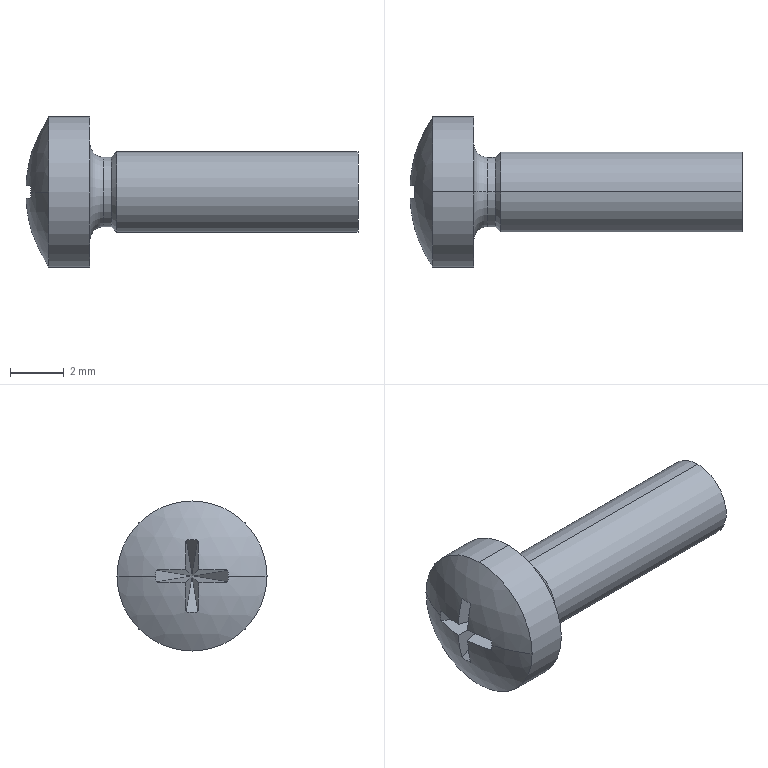Part | SolidWorks | features BaseBody 1 | 1 solid | 26 faces | box 12.388 x 5.6 x 5.6 mm | volume 116.992 mm3 | plane 14 | cylinder 6 | cone 2 | torus 2 | sphere 2 | commonest cylinder face diameters 2.598 x2 3 x2 5.6 x2
STEP:
#1=CARTESIAN_POINT('',(12.4,0.,1.5));
#2=VERTEX_POINT('',#1);
#3=CARTESIAN_POINT('',(12.4,0.,-1.5));
#4=VERTEX_POINT('',#3);
#5=CARTESIAN_POINT('',(12.4,0.,0.));
#6=DIRECTION('',(-1.,0.,0.));
#7=DIRECTION('',(0.,0.,1.));
#8=AXIS2_PLACEMENT_3D('',#5,#6,#7);
#9=CIRCLE('',#8,1.5);
#10=EDGE_CURVE('',#2,#4,#9,.T.);
#11=ORIENTED_EDGE('',*,*,#10,.T.);
#12=CARTESIAN_POINT('',(3.4,0.,-1.5));
#13=VERTEX_POINT('',#12);
#14=CARTESIAN_POINT('',(-1.332,0.,-1.5));
#15=DIRECTION('',(-1.,0.,0.));
#16=VECTOR('',#15,1000.);
#17=LINE('',#14,#16);
#18=EDGE_CURVE('',#4,#13,#17,.T.);
#19=ORIENTED_EDGE('',*,*,#18,.T.);
#20=CARTESIAN_POINT('',(3.4,0.,1.5));
#21=VERTEX_POINT('',#20);
#22=CARTESIAN_POINT('',(3.4,0.,0.));
#23=DIRECTION('',(-1.,0.,0.));
#24=DIRECTION('',(0.,0.,1.));
#25=AXIS2_PLACEMENT_3D('',#22,#23,#24);
#26=CIRCLE('',#25,1.5);
#27=EDGE_CURVE('',#21,#13,#26,.T.);
#28=ORIENTED_EDGE('',*,*,#27,.F.);
#29=CARTESIAN_POINT('',(-1.332,0.,1.5));
#30=DIRECTION('',(-1.,0.,0.));
#31=VECTOR('',#30,1000.);
#32=LINE('',#29,#31);
#33=EDGE_CURVE('',#2,#21,#32,.T.);
#34=ORIENTED_EDGE('',*,*,#33,.F.);
#35=EDGE_LOOP('',(#11,#19,#28,#34));
#36=FACE_OUTER_BOUND('',#35,.T.);
#37=CARTESIAN_POINT('',(-1.332,0.,0.));
#38=DIRECTION('',(-1.,0.,0.));
#39=DIRECTION('',(0.,0.,1.));
#40=AXIS2_PLACEMENT_3D('',#37,#38,#39);
#41=CYLINDRICAL_SURFACE('',#40,1.5);
#42=ADVANCED_FACE('',(#36),#41,.T.);
#43=CARTESIAN_POINT('',(3.199,0.,1.299));
#44=VERTEX_POINT('',#43);
#45=CARTESIAN_POINT('',(3.199,0.,-1.299));
#46=VERTEX_POINT('',#45);
#47=CARTESIAN_POINT('',(3.199,0.,0.));
#48=DIRECTION('',(-1.,0.,0.));
#49=DIRECTION('',(0.,0.,1.));
#50=AXIS2_PLACEMENT_3D('',#47,#48,#49);
#51=CIRCLE('',#50,1.299);
#52=EDGE_CURVE('',#44,#46,#51,.T.);
#53=ORIENTED_EDGE('',*,*,#52,.F.);
#54=CARTESIAN_POINT('',(3.4,0.,1.5));
#55=DIRECTION('',(0.7071,0.,0.7071));
#56=VECTOR('',#55,1000.);
#57=LINE('',#54,#56);
#58=EDGE_CURVE('',#44,#21,#57,.T.);
#59=ORIENTED_EDGE('',*,*,#58,.T.);
#60=ORIENTED_EDGE('',*,*,#27,.T.);
#61=CARTESIAN_POINT('',(3.4,0.,-1.5));
#62=DIRECTION('',(0.7071,0.,-0.7071));
#63=VECTOR('',#62,1000.);
#64=LINE('',#61,#63);
#65=EDGE_CURVE('',#46,#13,#64,.T.);
#66=ORIENTED_EDGE('',*,*,#65,.F.);
#67=EDGE_LOOP('',(#53,#59,#60,#66));
#68=FACE_OUTER_BOUND('',#67,.T.);
#69=CARTESIAN_POINT('',(3.4,0.,0.));
#70=DIRECTION('',(1.,0.,0.));
#71=DIRECTION('',(0.,0.,-1.));
#72=AXIS2_PLACEMENT_3D('',#69,#70,#71);
#73=CONICAL_SURFACE('',#72,1.5,0.7854);
#74=ADVANCED_FACE('',(#68),#73,.T.);
#75=ORIENTED_EDGE('',*,*,#52,.T.);
#76=CARTESIAN_POINT('',(2.901,0.,-1.299));
#77=VERTEX_POINT('',#76);
#78=CARTESIAN_POINT('',(-1.332,0.,-1.299));
#79=DIRECTION('',(-1.,0.,0.));
#80=VECTOR('',#79,1000.);
#81=LINE('',#78,#80);
#82=EDGE_CURVE('',#46,#77,#81,.T.);
#83=ORIENTED_EDGE('',*,*,#82,.T.);
#84=CARTESIAN_POINT('',(2.901,0.,1.299));
#85=VERTEX_POINT('',#84);
#86=CARTESIAN_POINT('',(2.901,0.,0.));
#87=DIRECTION('',(-1.,0.,0.));
#88=DIRECTION('',(0.,0.,1.));
#89=AXIS2_PLACEMENT_3D('',#86,#87,#88);
#90=CIRCLE('',#89,1.299);
#91=EDGE_CURVE('',#85,#77,#90,.T.);
#92=ORIENTED_EDGE('',*,*,#91,.F.);
#93=CARTESIAN_POINT('',(-1.332,0.,1.299));
#94=DIRECTION('',(-1.,0.,0.));
#95=VECTOR('',#94,1000.);
#96=LINE('',#93,#95);
#97=EDGE_CURVE('',#44,#85,#96,.T.);
#98=ORIENTED_EDGE('',*,*,#97,.F.);
#99=EDGE_LOOP('',(#75,#83,#92,#98));
#100=FACE_OUTER_BOUND('',#99,.T.);
#101=CARTESIAN_POINT('',(-1.332,0.,0.));
#102=DIRECTION('',(-1.,0.,0.));
#103=DIRECTION('',(0.,0.,1.));
#104=AXIS2_PLACEMENT_3D('',#101,#102,#103);
#105=CYLINDRICAL_SURFACE('',#104,1.299);
#106=ADVANCED_FACE('',(#100),#105,.T.);
#107=CARTESIAN_POINT('',(2.4,0.,-1.8));
#108=VERTEX_POINT('',#107);
#109=CARTESIAN_POINT('',(2.4,0.,1.8));
#110=VERTEX_POINT('',#109);
#111=CARTESIAN_POINT('',(2.4,0.,0.));
#112=DIRECTION('',(-1.,0.,0.));
#113=DIRECTION('',(0.,0.,1.));
#114=AXIS2_PLACEMENT_3D('',#111,#112,#113);
#115=CIRCLE('',#114,1.8);
#116=EDGE_CURVE('',#108,#110,#115,.T.);
#117=ORIENTED_EDGE('',*,*,#116,.F.);
#118=CARTESIAN_POINT('',(2.901,0.,-1.8));
#119=DIRECTION('',(0.,1.,0.));
#120=DIRECTION('',(0.,0.,1.));
#121=AXIS2_PLACEMENT_3D('',#118,#119,#120);
#122=CIRCLE('',#121,0.501);
#123=EDGE_CURVE('',#108,#77,#122,.T.);
#124=ORIENTED_EDGE('',*,*,#123,.T.);
#125=CARTESIAN_POINT('',(2.901,0.,0.));
#126=DIRECTION('',(-1.,0.,0.));
#127=DIRECTION('',(0.,0.,1.));
#128=AXIS2_PLACEMENT_3D('',#125,#126,#127);
#129=CIRCLE('',#128,1.299);
#130=EDGE_CURVE('',#77,#85,#129,.T.);
#131=ORIENTED_EDGE('',*,*,#130,.T.);
#132=CARTESIAN_POINT('',(2.901,0.,1.8));
#133=DIRECTION('',(0.,-1.,0.));
#134=DIRECTION('',(0.,0.,-1.));
#135=AXIS2_PLACEMENT_3D('',#132,#133,#134);
#136=CIRCLE('',#135,0.501);
#137=EDGE_CURVE('',#110,#85,#136,.T.);
#138=ORIENTED_EDGE('',*,*,#137,.F.);
#139=EDGE_LOOP('',(#117,#124,#131,#138));
#140=FACE_OUTER_BOUND('',#139,.T.);
#141=CARTESIAN_POINT('',(2.901,0.,0.));
#142=DIRECTION('',(-1.,0.,0.));
#143=DIRECTION('',(0.,0.,1.));
#144=AXIS2_PLACEMENT_3D('',#141,#142,#143);
#145=TOROIDAL_SURFACE('',#144,1.8,0.501);
#146=ADVANCED_FACE('',(#140),#145,.F.);
#147=CARTESIAN_POINT('',(2.4,0.,2.8));
#148=VERTEX_POINT('',#147);
#149=CARTESIAN_POINT('',(2.4,0.,-2.8));
#150=VERTEX_POINT('',#149);
#151=CARTESIAN_POINT('',(2.4,0.,0.));
#152=DIRECTION('',(-1.,0.,0.));
#153=DIRECTION('',(0.,0.,1.));
#154=AXIS2_PLACEMENT_3D('',#151,#152,#153);
#155=CIRCLE('',#154,2.8);
#156=EDGE_CURVE('',#148,#150,#155,.T.);
#157=ORIENTED_EDGE('',*,*,#156,.T.);
#158=CARTESIAN_POINT('',(0.8575,0.,-2.8));
#159=VERTEX_POINT('',#158);
#160=CARTESIAN_POINT('',(-1.332,0.,-2.8));
#161=DIRECTION('',(-1.,0.,0.));
#162=VECTOR('',#161,1000.);
#163=LINE('',#160,#162);
#164=EDGE_CURVE('',#150,#159,#163,.T.);
#165=ORIENTED_EDGE('',*,*,#164,.T.);
#166=CARTESIAN_POINT('',(0.8575,2.8,0.));
#167=VERTEX_POINT('',#166);
#168=CARTESIAN_POINT('',(0.8575,0.,0.));
#169=DIRECTION('',(-1.,0.,0.));
#170=DIRECTION('',(0.,0.,1.));
#171=AXIS2_PLACEMENT_3D('',#168,#169,#170);
#172=CIRCLE('',#171,2.8);
#173=EDGE_CURVE('',#167,#159,#172,.T.);
#174=ORIENTED_EDGE('',*,*,#173,.F.);
#175=CARTESIAN_POINT('',(0.8575,0.,2.8));
#176=VERTEX_POINT('',#175);
#177=CARTESIAN_POINT('',(0.8575,0.,0.));
#178=DIRECTION('',(-1.,0.,0.));
#179=DIRECTION('',(0.,0.,1.));
#180=AXIS2_PLACEMENT_3D('',#177,#178,#179);
#181=CIRCLE('',#180,2.8);
#182=EDGE_CURVE('',#176,#167,#181,.T.);
#183=ORIENTED_EDGE('',*,*,#182,.F.);
#184=CARTESIAN_POINT('',(-1.332,0.,2.8));
#185=DIRECTION('',(-1.,0.,0.));
#186=VECTOR('',#185,1000.);
#187=LINE('',#184,#186);
#188=EDGE_CURVE('',#148,#176,#187,.T.);
#189=ORIENTED_EDGE('',*,*,#188,.F.);
#190=EDGE_LOOP('',(#157,#165,#174,#183,#189));
#191=FACE_OUTER_BOUND('',#190,.T.);
#192=CARTESIAN_POINT('',(-1.332,0.,0.));
#193=DIRECTION('',(-1.,0.,0.));
#194=DIRECTION('',(0.,0.,1.));
#195=AXIS2_PLACEMENT_3D('',#192,#193,#194);
#196=CYLINDRICAL_SURFACE('',#195,2.8);
#197=ADVANCED_FACE('',(#191),#196,.T.);
#198=ORIENTED_EDGE('',*,*,#173,.T.);
#199=CARTESIAN_POINT('',(0.8575,-2.8,0.));
#200=VERTEX_POINT('',#199);
#201=CARTESIAN_POINT('',(0.8575,0.,0.));
#202=DIRECTION('',(-1.,0.,0.));
#203=DIRECTION('',(0.,0.,1.));
#204=AXIS2_PLACEMENT_3D('',#201,#202,#203);
#205=CIRCLE('',#204,2.8);
#206=EDGE_CURVE('',#159,#200,#205,.T.);
#207=ORIENTED_EDGE('',*,*,#206,.T.);
#208=CARTESIAN_POINT('',(0.1846,-1.346,0.));
#209=VERTEX_POINT('',#208);
#210=CARTESIAN_POINT('',(5.,0.,0.));
#211=DIRECTION('',(0.,0.,-1.));
#212=DIRECTION('',(0.,1.,0.));
#213=AXIS2_PLACEMENT_3D('',#210,#211,#212);
#214=CIRCLE('',#213,5.);
#215=EDGE_CURVE('',#200,#209,#214,.T.);
#216=ORIENTED_EDGE('',*,*,#215,.T.);
#217=CARTESIAN_POINT('',(0.1888,-1.343,-0.2238));
#218=VERTEX_POINT('',#217);
#219=CARTESIAN_POINT('',(3.689,1.574,0.));
#220=DIRECTION('',(0.6402,-0.7682,0.));
#221=DIRECTION('',(0.7682,0.6402,0.));
#222=AXIS2_PLACEMENT_3D('',#219,#220,#221);
#223=CIRCLE('',#222,4.561);
#224=EDGE_CURVE('',#209,#218,#223,.T.);
#225=ORIENTED_EDGE('',*,*,#224,.T.);
#226=CARTESIAN_POINT('',(0.01234,-0.2483,-0.2483));
#227=VERTEX_POINT('',#226);
#228=CARTESIAN_POINT('',(4.939,0.,0.436));
#229=DIRECTION('',(0.1376,0.,-0.9905));
#230=DIRECTION('',(-0.9905,0.,-0.1376));
#231=AXIS2_PLACEMENT_3D('',#228,#229,#230);
#232=CIRCLE('',#231,4.981);
#233=EDGE_CURVE('',#218,#227,#232,.T.);
#234=ORIENTED_EDGE('',*,*,#233,.T.);
#235=CARTESIAN_POINT('',(0.1888,-0.2238,-1.343));
#236=VERTEX_POINT('',#235);
#237=CARTESIAN_POINT('',(4.939,0.436,0.));
#238=DIRECTION('',(0.1376,-0.9905,0.));
#239=DIRECTION('',(0.9905,0.1376,0.));
#240=AXIS2_PLACEMENT_3D('',#237,#238,#239);
#241=CIRCLE('',#240,4.981);
#242=EDGE_CURVE('',#227,#236,#241,.T.);
#243=ORIENTED_EDGE('',*,*,#242,.T.);
#244=CARTESIAN_POINT('',(0.1888,0.2238,-1.343));
#245=VERTEX_POINT('',#244);
#246=CARTESIAN_POINT('',(3.689,0.,1.574));
#247=DIRECTION('',(0.6402,0.,-0.7682));
#248=DIRECTION('',(-0.7682,0.,-0.6402));
#249=AXIS2_PLACEMENT_3D('',#246,#247,#248);
#250=CIRCLE('',#249,4.561);
#251=EDGE_CURVE('',#236,#245,#250,.T.);
#252=ORIENTED_EDGE('',*,*,#251,.T.);
#253=CARTESIAN_POINT('',(0.01234,0.2483,-0.2483));
#254=VERTEX_POINT('',#253);
#255=CARTESIAN_POINT('',(4.939,-0.436,0.));
#256=DIRECTION('',(0.1376,0.9905,0.));
#257=DIRECTION('',(-0.9905,0.1376,0.));
#258=AXIS2_PLACEMENT_3D('',#255,#256,#257);
#259=CIRCLE('',#258,4.981);
#260=EDGE_CURVE('',#245,#254,#259,.T.);
#261=ORIENTED_EDGE('',*,*,#260,.T.);
#262=CARTESIAN_POINT('',(0.1888,1.343,-0.2238));
#263=VERTEX_POINT('',#262);
#264=CARTESIAN_POINT('',(4.939,0.,0.436));
#265=DIRECTION('',(0.1376,0.,-0.9905));
#266=DIRECTION('',(-0.9905,0.,-0.1376));
#267=AXIS2_PLACEMENT_3D('',#264,#265,#266);
#268=CIRCLE('',#267,4.981);
#269=EDGE_CURVE('',#254,#263,#268,.T.);
#270=ORIENTED_EDGE('',*,*,#269,.T.);
#271=CARTESIAN_POINT('',(0.1846,1.346,0.));
#272=VERTEX_POINT('',#271);
#273=CARTESIAN_POINT('',(3.689,-1.574,0.));
#274=DIRECTION('',(0.6402,0.7682,0.));
#275=DIRECTION('',(-0.7682,0.6402,0.));
#276=AXIS2_PLACEMENT_3D('',#273,#274,#275);
#277=CIRCLE('',#276,4.561);
#278=EDGE_CURVE('',#263,#272,#277,.T.);
#279=ORIENTED_EDGE('',*,*,#278,.T.);
#280=CARTESIAN_POINT('',(5.,0.,0.));
#281=DIRECTION('',(0.,0.,1.));
#282=DIRECTION('',(1.,0.,0.));
#283=AXIS2_PLACEMENT_3D('',#280,#281,#282);
#284=CIRCLE('',#283,5.);
#285=EDGE_CURVE('',#167,#272,#284,.T.);
#286=ORIENTED_EDGE('',*,*,#285,.F.);
#287=EDGE_LOOP('',(#198,#207,#216,#225,#234,#243,#252,#261,#270,#279,#286));
#288=FACE_OUTER_BOUND('',#287,.T.);
#289=CARTESIAN_POINT('',(5.,0.,0.));
#290=DIRECTION('',(0.,0.,-1.));
#291=DIRECTION('',(0.,1.,0.));
#292=AXIS2_PLACEMENT_3D('',#289,#290,#291);
#293=SPHERICAL_SURFACE('',#292,5.);
#294=ADVANCED_FACE('',(#288),#293,.T.);
#295=CARTESIAN_POINT('',(1.8,0.,0.));
#296=VERTEX_POINT('',#295);
#297=CARTESIAN_POINT('',(1.8,0.,0.));
#298=DIRECTION('',(-0.7639,-0.6366,-0.1061));
#299=VECTOR('',#298,1000.);
#300=LINE('',#297,#299);
#301=EDGE_CURVE('',#296,#218,#300,.T.);
#302=ORIENTED_EDGE('',*,*,#301,.F.);
#303=CARTESIAN_POINT('',(1.8,0.,0.));
#304=DIRECTION('',(-0.9813,-0.1363,-0.1363));
#305=VECTOR('',#304,1000.);
#306=LINE('',#303,#305);
#307=EDGE_CURVE('',#296,#227,#306,.T.);
#308=ORIENTED_EDGE('',*,*,#307,.T.);
#309=ORIENTED_EDGE('',*,*,#233,.F.);
#310=EDGE_LOOP('',(#302,#308,#309));
#311=FACE_OUTER_BOUND('',#310,.T.);
#312=CARTESIAN_POINT('',(1.8,0.,0.));
#313=DIRECTION('',(0.1376,0.,-0.9905));
#314=DIRECTION('',(-0.9905,0.,-0.1376));
#315=AXIS2_PLACEMENT_3D('',#312,#313,#314);
#316=PLANE('',#315);
#317=ADVANCED_FACE('',(#311),#316,.F.);
#318=CARTESIAN_POINT('',(0.01234,-0.2483,0.2483));
#319=VERTEX_POINT('',#318);
#320=CARTESIAN_POINT('',(0.1888,-1.343,0.2238));
#321=VERTEX_POINT('',#320);
#322=CARTESIAN_POINT('',(4.939,0.,-0.436));
#323=DIRECTION('',(0.1376,0.,0.9905));
#324=DIRECTION('',(0.9905,0.,-0.1376));
#325=AXIS2_PLACEMENT_3D('',#322,#323,#324);
#326=CIRCLE('',#325,4.981);
#327=EDGE_CURVE('',#319,#321,#326,.T.);
#328=ORIENTED_EDGE('',*,*,#327,.F.);
#329=CARTESIAN_POINT('',(1.8,0.,0.));
#330=DIRECTION('',(0.9813,0.1363,-0.1363));
#331=VECTOR('',#330,1000.);
#332=LINE('',#329,#331);
#333=EDGE_CURVE('',#319,#296,#332,.T.);
#334=ORIENTED_EDGE('',*,*,#333,.T.);
#335=CARTESIAN_POINT('',(1.8,0.,0.));
#336=DIRECTION('',(-0.7639,-0.6366,0.1061));
#337=VECTOR('',#336,1000.);
#338=LINE('',#335,#337);
#339=EDGE_CURVE('',#296,#321,#338,.T.);
#340=ORIENTED_EDGE('',*,*,#339,.T.);
#341=EDGE_LOOP('',(#328,#334,#340));
#342=FACE_OUTER_BOUND('',#341,.T.);
#343=CARTESIAN_POINT('',(1.8,0.,0.));
#344=DIRECTION('',(0.1376,0.,0.9905));
#345=DIRECTION('',(0.9905,0.,-0.1376));
#346=AXIS2_PLACEMENT_3D('',#343,#344,#345);
#347=PLANE('',#346);
#348=ADVANCED_FACE('',(#342),#347,.F.);
#349=ORIENTED_EDGE('',*,*,#215,.F.);
#350=CARTESIAN_POINT('',(0.8575,0.,0.));
#351=DIRECTION('',(-1.,0.,0.));
#352=DIRECTION('',(0.,0.,1.));
#353=AXIS2_PLACEMENT_3D('',#350,#351,#352);
#354=CIRCLE('',#353,2.8);
#355=EDGE_CURVE('',#200,#176,#354,.T.);
#356=ORIENTED_EDGE('',*,*,#355,.T.);
#357=ORIENTED_EDGE('',*,*,#182,.T.);
#358=ORIENTED_EDGE('',*,*,#285,.T.);
#359=CARTESIAN_POINT('',(0.1888,1.343,0.2238));
#360=VERTEX_POINT('',#359);
#361=CARTESIAN_POINT('',(3.689,-1.574,0.));
#362=DIRECTION('',(0.6402,0.7682,0.));
#363=DIRECTION('',(-0.7682,0.6402,0.));
#364=AXIS2_PLACEMENT_3D('',#361,#362,#363);
#365=CIRCLE('',#364,4.561);
#366=EDGE_CURVE('',#272,#360,#365,.T.);
#367=ORIENTED_EDGE('',*,*,#366,.T.);
#368=CARTESIAN_POINT('',(0.01234,0.2483,0.2483));
#369=VERTEX_POINT('',#368);
#370=CARTESIAN_POINT('',(4.939,0.,-0.436));
#371=DIRECTION('',(0.1376,0.,0.9905));
#372=DIRECTION('',(0.9905,0.,-0.1376));
#373=AXIS2_PLACEMENT_3D('',#370,#371,#372);
#374=CIRCLE('',#373,4.981);
#375=EDGE_CURVE('',#360,#369,#374,.T.);
#376=ORIENTED_EDGE('',*,*,#375,.T.);
#377=CARTESIAN_POINT('',(0.1888,0.2238,1.343));
#378=VERTEX_POINT('',#377);
#379=CARTESIAN_POINT('',(4.939,-0.436,0.));
#380=DIRECTION('',(0.1376,0.9905,0.));
#381=DIRECTION('',(-0.9905,0.1376,0.));
#382=AXIS2_PLACEMENT_3D('',#379,#380,#381);
#383=CIRCLE('',#382,4.981);
#384=EDGE_CURVE('',#369,#378,#383,.T.);
#385=ORIENTED_EDGE('',*,*,#384,.T.);
#386=CARTESIAN_POINT('',(0.1888,-0.2238,1.343));
#387=VERTEX_POINT('',#386);
#388=CARTESIAN_POINT('',(3.689,0.,-1.574));
#389=DIRECTION('',(0.6402,0.,0.7682));
#390=DIRECTION('',(0.7682,0.,-0.6402));
#391=AXIS2_PLACEMENT_3D('',#388,#389,#390);
#392=CIRCLE('',#391,4.561);
#393=EDGE_CURVE('',#378,#387,#392,.T.);
#394=ORIENTED_EDGE('',*,*,#393,.T.);
#395=CARTESIAN_POINT('',(4.939,0.436,0.));
#396=DIRECTION('',(0.1376,-0.9905,0.));
#397=DIRECTION('',(0.9905,0.1376,0.));
#398=AXIS2_PLACEMENT_3D('',#395,#396,#397);
#399=CIRCLE('',#398,4.981);
#400=EDGE_CURVE('',#387,#319,#399,.T.);
#401=ORIENTED_EDGE('',*,*,#400,.T.);
#402=ORIENTED_EDGE('',*,*,#327,.T.);
#403=CARTESIAN_POINT('',(3.689,1.574,0.));
#404=DIRECTION('',(0.6402,-0.7682,0.));
#405=DIRECTION('',(0.7682,0.6402,0.));
#406=AXIS2_PLACEMENT_3D('',#403,#404,#405);
#407=CIRCLE('',#406,4.561);
#408=EDGE_CURVE('',#321,#209,#407,.T.);
#409=ORIENTED_EDGE('',*,*,#408,.T.);
#410=EDGE_LOOP('',(#349,#356,#357,#358,#367,#376,#385,#394,#401,#402,#409));
#411=FACE_OUTER_BOUND('',#410,.T.);
#412=CARTESIAN_POINT('',(5.,0.,0.));
#413=DIRECTION('',(0.,0.,-1.));
#414=DIRECTION('',(0.,1.,0.));
#415=AXIS2_PLACEMENT_3D('',#412,#413,#414);
#416=SPHERICAL_SURFACE('',#415,5.);
#417=ADVANCED_FACE('',(#411),#416,.T.);
#418=ORIENTED_EDGE('',*,*,#164,.F.);
#419=CARTESIAN_POINT('',(2.4,0.,0.));
#420=DIRECTION('',(-1.,0.,0.));
#421=DIRECTION('',(0.,0.,1.));
#422=AXIS2_PLACEMENT_3D('',#419,#420,#421);
#423=CIRCLE('',#422,2.8);
#424=EDGE_CURVE('',#150,#148,#423,.T.);
#425=ORIENTED_EDGE('',*,*,#424,.T.);
#426=ORIENTED_EDGE('',*,*,#188,.T.);
#427=ORIENTED_EDGE('',*,*,#355,.F.);
#428=ORIENTED_EDGE('',*,*,#206,.F.);
#429=EDGE_LOOP('',(#418,#425,#426,#427,#428));
#430=FACE_OUTER_BOUND('',#429,.T.);
#431=CARTESIAN_POINT('',(-1.332,0.,0.));
#432=DIRECTION('',(-1.,0.,0.));
#433=DIRECTION('',(0.,0.,1.));
#434=AXIS2_PLACEMENT_3D('',#431,#432,#433);
#435=CYLINDRICAL_SURFACE('',#434,2.8);
#436=ADVANCED_FACE('',(#430),#435,.T.);
#437=ORIENTED_EDGE('',*,*,#156,.F.);
#438=ORIENTED_EDGE('',*,*,#424,.F.);
#439=EDGE_LOOP('',(#437,#438));
#440=FACE_OUTER_BOUND('',#439,.T.);
#441=CARTESIAN_POINT('',(2.4,0.,0.));
#442=DIRECTION('',(-1.,0.,0.));
#443=DIRECTION('',(0.,0.,1.));
#444=AXIS2_PLACEMENT_3D('',#441,#442,#443);
#445=CIRCLE('',#444,1.8);
#446=EDGE_CURVE('',#110,#108,#445,.T.);
#447=ORIENTED_EDGE('',*,*,#446,.T.);
#448=ORIENTED_EDGE('',*,*,#116,.T.);
#449=EDGE_LOOP('',(#447,#448));
#450=FACE_BOUND('',#449,.T.);
#451=CARTESIAN_POINT('',(2.4,1.8,0.));
#452=DIRECTION('',(-1.,0.,0.));
#453=DIRECTION('',(0.,0.,1.));
#454=AXIS2_PLACEMENT_3D('',#451,#452,#453);
#455=PLANE('',#454);
#456=ADVANCED_FACE('',(#440,#450),#455,.F.);
#457=ORIENTED_EDGE('',*,*,#123,.F.);
#458=ORIENTED_EDGE('',*,*,#446,.F.);
#459=ORIENTED_EDGE('',*,*,#137,.T.);
#460=ORIENTED_EDGE('',*,*,#91,.T.);
#461=EDGE_LOOP('',(#457,#458,#459,#460));
#462=FACE_OUTER_BOUND('',#461,.T.);
#463=CARTESIAN_POINT('',(2.901,0.,0.));
#464=DIRECTION('',(-1.,0.,0.));
#465=DIRECTION('',(0.,0.,1.));
#466=AXIS2_PLACEMENT_3D('',#463,#464,#465);
#467=TOROIDAL_SURFACE('',#466,1.8,0.501);
#468=ADVANCED_FACE('',(#462),#467,.F.);
#469=ORIENTED_EDGE('',*,*,#82,.F.);
#470=CARTESIAN_POINT('',(3.199,0.,0.));
#471=DIRECTION('',(-1.,0.,0.));
#472=DIRECTION('',(0.,0.,1.));
#473=AXIS2_PLACEMENT_3D('',#470,#471,#472);
#474=CIRCLE('',#473,1.299);
#475=EDGE_CURVE('',#46,#44,#474,.T.);
#476=ORIENTED_EDGE('',*,*,#475,.T.);
#477=ORIENTED_EDGE('',*,*,#97,.T.);
#478=ORIENTED_EDGE('',*,*,#130,.F.);
#479=EDGE_LOOP('',(#469,#476,#477,#478));
#480=FACE_OUTER_BOUND('',#479,.T.);
#481=CARTESIAN_POINT('',(-1.332,0.,0.));
#482=DIRECTION('',(-1.,0.,0.));
#483=DIRECTION('',(0.,0.,1.));
#484=AXIS2_PLACEMENT_3D('',#481,#482,#483);
#485=CYLINDRICAL_SURFACE('',#484,1.299);
#486=ADVANCED_FACE('',(#480),#485,.T.);
#487=ORIENTED_EDGE('',*,*,#58,.F.);
#488=ORIENTED_EDGE('',*,*,#475,.F.);
#489=ORIENTED_EDGE('',*,*,#65,.T.);
#490=CARTESIAN_POINT('',(3.4,0.,0.));
#491=DIRECTION('',(-1.,0.,0.));
#492=DIRECTION('',(0.,0.,1.));
#493=AXIS2_PLACEMENT_3D('',#490,#491,#492);
#494=CIRCLE('',#493,1.5);
#495=EDGE_CURVE('',#13,#21,#494,.T.);
#496=ORIENTED_EDGE('',*,*,#495,.T.);
#497=EDGE_LOOP('',(#487,#488,#489,#496));
#498=FACE_OUTER_BOUND('',#497,.T.);
#499=CARTESIAN_POINT('',(3.4,0.,0.));
#500=DIRECTION('',(1.,0.,0.));
#501=DIRECTION('',(0.,0.,-1.));
#502=AXIS2_PLACEMENT_3D('',#499,#500,#501);
#503=CONICAL_SURFACE('',#502,1.5,0.7854);
#504=ADVANCED_FACE('',(#498),#503,.T.);
#505=ORIENTED_EDGE('',*,*,#18,.F.);
#506=CARTESIAN_POINT('',(12.4,0.,0.));
#507=DIRECTION('',(-1.,0.,0.));
#508=DIRECTION('',(0.,0.,1.));
#509=AXIS2_PLACEMENT_3D('',#506,#507,#508);
#510=CIRCLE('',#509,1.5);
#511=EDGE_CURVE('',#4,#2,#510,.T.);
#512=ORIENTED_EDGE('',*,*,#511,.T.);
#513=ORIENTED_EDGE('',*,*,#33,.T.);
#514=ORIENTED_EDGE('',*,*,#495,.F.);
#515=EDGE_LOOP('',(#505,#512,#513,#514));
#516=FACE_OUTER_BOUND('',#515,.T.);
#517=CARTESIAN_POINT('',(-1.332,0.,0.));
#518=DIRECTION('',(-1.,0.,0.));
#519=DIRECTION('',(0.,0.,1.));
#520=AXIS2_PLACEMENT_3D('',#517,#518,#519);
#521=CYLINDRICAL_SURFACE('',#520,1.5);
#522=ADVANCED_FACE('',(#516),#521,.T.);
#523=ORIENTED_EDGE('',*,*,#10,.F.);
#524=ORIENTED_EDGE('',*,*,#511,.F.);
#525=EDGE_LOOP('',(#523,#524));
#526=FACE_OUTER_BOUND('',#525,.T.);
#527=CARTESIAN_POINT('',(12.4,0.,0.));
#528=DIRECTION('',(-1.,0.,0.));
#529=DIRECTION('',(0.,0.,1.));
#530=AXIS2_PLACEMENT_3D('',#527,#528,#529);
#531=PLANE('',#530);
#532=ADVANCED_FACE('',(#526),#531,.F.);
#533=ORIENTED_EDGE('',*,*,#269,.F.);
#534=CARTESIAN_POINT('',(1.8,0.,0.));
#535=DIRECTION('',(0.9813,-0.1363,0.1363));
#536=VECTOR('',#535,1000.);
#537=LINE('',#534,#536);
#538=EDGE_CURVE('',#254,#296,#537,.T.);
#539=ORIENTED_EDGE('',*,*,#538,.T.);
#540=CARTESIAN_POINT('',(1.8,0.,0.));
#541=DIRECTION('',(-0.7639,0.6366,-0.1061));
#542=VECTOR('',#541,1000.);
#543=LINE('',#540,#542);
#544=EDGE_CURVE('',#296,#263,#543,.T.);
#545=ORIENTED_EDGE('',*,*,#544,.T.);
#546=EDGE_LOOP('',(#533,#539,#545));
#547=FACE_OUTER_BOUND('',#546,.T.);
#548=CARTESIAN_POINT('',(1.8,0.,0.));
#549=DIRECTION('',(0.1376,0.,-0.9905));
#550=DIRECTION('',(-0.9905,0.,-0.1376));
#551=AXIS2_PLACEMENT_3D('',#548,#549,#550);
#552=PLANE('',#551);
#553=ADVANCED_FACE('',(#547),#552,.F.);
#554=ORIENTED_EDGE('',*,*,#544,.F.);
#555=CARTESIAN_POINT('',(1.8,0.,0.));
#556=DIRECTION('',(-0.7639,0.6366,0.1061));
#557=VECTOR('',#556,1000.);
#558=LINE('',#555,#557);
#559=EDGE_CURVE('',#296,#360,#558,.T.);
#560=ORIENTED_EDGE('',*,*,#559,.T.);
#561=ORIENTED_EDGE('',*,*,#366,.F.);
#562=ORIENTED_EDGE('',*,*,#278,.F.);
#563=EDGE_LOOP('',(#554,#560,#561,#562));
#564=FACE_OUTER_BOUND('',#563,.T.);
#565=CARTESIAN_POINT('',(0.,1.5,-0.25));
#566=DIRECTION('',(0.6402,0.7682,0.));
#567=DIRECTION('',(-0.7682,0.6402,0.));
#568=AXIS2_PLACEMENT_3D('',#565,#566,#567);
#569=PLANE('',#568);
#570=ADVANCED_FACE('',(#564),#569,.F.);
#571=ORIENTED_EDGE('',*,*,#339,.F.);
#572=ORIENTED_EDGE('',*,*,#301,.T.);
#573=ORIENTED_EDGE('',*,*,#224,.F.);
#574=ORIENTED_EDGE('',*,*,#408,.F.);
#575=EDGE_LOOP('',(#571,#572,#573,#574));
#576=FACE_OUTER_BOUND('',#575,.T.);
#577=CARTESIAN_POINT('',(0.,-1.5,0.25));
#578=DIRECTION('',(0.6402,-0.7682,0.));
#579=DIRECTION('',(0.7682,0.6402,0.));
#580=AXIS2_PLACEMENT_3D('',#577,#578,#579);
#581=PLANE('',#580);
#582=ADVANCED_FACE('',(#576),#581,.F.);
#583=ORIENTED_EDGE('',*,*,#559,.F.);
#584=CARTESIAN_POINT('',(1.8,0.,0.));
#585=DIRECTION('',(-0.9813,0.1363,0.1363));
#586=VECTOR('',#585,1000.);
#587=LINE('',#584,#586);
#588=EDGE_CURVE('',#296,#369,#587,.T.);
#589=ORIENTED_EDGE('',*,*,#588,.T.);
#590=ORIENTED_EDGE('',*,*,#375,.F.);
#591=EDGE_LOOP('',(#583,#589,#590));
#592=FACE_OUTER_BOUND('',#591,.T.);
#593=CARTESIAN_POINT('',(1.8,0.,0.));
#594=DIRECTION('',(0.1376,0.,0.9905));
#595=DIRECTION('',(0.9905,0.,-0.1376));
#596=AXIS2_PLACEMENT_3D('',#593,#594,#595);
#597=PLANE('',#596);
#598=ADVANCED_FACE('',(#592),#597,.F.);
#599=CARTESIAN_POINT('',(1.8,0.,0.));
#600=DIRECTION('',(-0.7639,-0.1061,0.6366));
#601=VECTOR('',#600,1000.);
#602=LINE('',#599,#601);
#603=EDGE_CURVE('',#296,#387,#602,.T.);
#604=ORIENTED_EDGE('',*,*,#603,.F.);
#605=ORIENTED_EDGE('',*,*,#333,.F.);
#606=ORIENTED_EDGE('',*,*,#400,.F.);
#607=EDGE_LOOP('',(#604,#605,#606));
#608=FACE_OUTER_BOUND('',#607,.T.);
#609=CARTESIAN_POINT('',(1.8,0.,0.));
#610=DIRECTION('',(0.1376,-0.9905,0.));
#611=DIRECTION('',(-0.9905,-0.1376,0.));
#612=AXIS2_PLACEMENT_3D('',#609,#610,#611);
#613=PLANE('',#612);
#614=ADVANCED_FACE('',(#608),#613,.F.);
#615=ORIENTED_EDGE('',*,*,#588,.F.);
#616=CARTESIAN_POINT('',(1.8,0.,0.));
#617=DIRECTION('',(-0.7639,0.1061,0.6366));
#618=VECTOR('',#617,1000.);
#619=LINE('',#616,#618);
#620=EDGE_CURVE('',#296,#378,#619,.T.);
#621=ORIENTED_EDGE('',*,*,#620,.T.);
#622=ORIENTED_EDGE('',*,*,#384,.F.);
#623=EDGE_LOOP('',(#615,#621,#622));
#624=FACE_OUTER_BOUND('',#623,.T.);
#625=CARTESIAN_POINT('',(1.8,0.,0.));
#626=DIRECTION('',(0.1376,0.9905,0.));
#627=DIRECTION('',(0.9905,-0.1376,0.));
#628=AXIS2_PLACEMENT_3D('',#625,#626,#627);
#629=PLANE('',#628);
#630=ADVANCED_FACE('',(#624),#629,.F.);
#631=ORIENTED_EDGE('',*,*,#620,.F.);
#632=ORIENTED_EDGE('',*,*,#603,.T.);
#633=ORIENTED_EDGE('',*,*,#393,.F.);
#634=EDGE_LOOP('',(#631,#632,#633));
#635=FACE_OUTER_BOUND('',#634,.T.);
#636=CARTESIAN_POINT('',(0.,-0.25,1.5));
#637=DIRECTION('',(0.6402,0.,0.7682));
#638=DIRECTION('',(-0.7682,0.,0.6402));
#639=AXIS2_PLACEMENT_3D('',#636,#637,#638);
#640=PLANE('',#639);
#641=ADVANCED_FACE('',(#635),#640,.F.);
#642=ORIENTED_EDGE('',*,*,#307,.F.);
#643=CARTESIAN_POINT('',(1.8,0.,0.));
#644=DIRECTION('',(-0.7639,-0.1061,-0.6366));
#645=VECTOR('',#644,1000.);
#646=LINE('',#643,#645);
#647=EDGE_CURVE('',#296,#236,#646,.T.);
#648=ORIENTED_EDGE('',*,*,#647,.T.);
#649=ORIENTED_EDGE('',*,*,#242,.F.);
#650=EDGE_LOOP('',(#642,#648,#649));
#651=FACE_OUTER_BOUND('',#650,.T.);
#652=CARTESIAN_POINT('',(1.8,0.,0.));
#653=DIRECTION('',(0.1376,-0.9905,0.));
#654=DIRECTION('',(-0.9905,-0.1376,0.));
#655=AXIS2_PLACEMENT_3D('',#652,#653,#654);
#656=PLANE('',#655);
#657=ADVANCED_FACE('',(#651),#656,.F.);
#658=ORIENTED_EDGE('',*,*,#647,.F.);
#659=CARTESIAN_POINT('',(1.8,0.,0.));
#660=DIRECTION('',(-0.7639,0.1061,-0.6366));
#661=VECTOR('',#660,1000.);
#662=LINE('',#659,#661);
#663=EDGE_CURVE('',#296,#245,#662,.T.);
#664=ORIENTED_EDGE('',*,*,#663,.T.);
#665=ORIENTED_EDGE('',*,*,#251,.F.);
#666=EDGE_LOOP('',(#658,#664,#665));
#667=FACE_OUTER_BOUND('',#666,.T.);
#668=CARTESIAN_POINT('',(0.,0.25,-1.5));
#669=DIRECTION('',(0.6402,0.,-0.7682));
#670=DIRECTION('',(0.7682,0.,0.6402));
#671=AXIS2_PLACEMENT_3D('',#668,#669,#670);
#672=PLANE('',#671);
#673=ADVANCED_FACE('',(#667),#672,.F.);
#674=ORIENTED_EDGE('',*,*,#663,.F.);
#675=ORIENTED_EDGE('',*,*,#538,.F.);
#676=ORIENTED_EDGE('',*,*,#260,.F.);
#677=EDGE_LOOP('',(#674,#675,#676));
#678=FACE_OUTER_BOUND('',#677,.T.);
#679=CARTESIAN_POINT('',(1.8,0.,0.));
#680=DIRECTION('',(0.1376,0.9905,0.));
#681=DIRECTION('',(0.9905,-0.1376,0.));
#682=AXIS2_PLACEMENT_3D('',#679,#680,#681);
#683=PLANE('',#682);
#684=ADVANCED_FACE('',(#678),#683,.F.);
#685=CLOSED_SHELL('',(#42,#74,#106,#146,#197,#294,#317,#348,#417,#436,#456,#468,#486,#504,#522,#532,#553,#570,#582,#598,#614,#630,#641,#657,#673,#684));
#686=MANIFOLD_SOLID_BREP('',#685);
#687=CARTESIAN_POINT('',(0.,0.,0.));
#688=DIRECTION('',(0.,0.,1.));
#689=DIRECTION('',(1.,0.,0.));
#690=AXIS2_PLACEMENT_3D('',#687,#688,#689);
#691=(LENGTH_UNIT()NAMED_UNIT(*)SI_UNIT(.MILLI.,.METRE.));
#692=UNCERTAINTY_MEASURE_WITH_UNIT(LENGTH_MEASURE(0.00001),#691,'','');
#693=(NAMED_UNIT(*)PLANE_ANGLE_UNIT()SI_UNIT($,.RADIAN.));
#694=(NAMED_UNIT(*)SI_UNIT($,.STERADIAN.)SOLID_ANGLE_UNIT());
#695=(GEOMETRIC_REPRESENTATION_CONTEXT(3)GLOBAL_UNCERTAINTY_ASSIGNED_CONTEXT((#692))GLOBAL_UNIT_ASSIGNED_CONTEXT((#691,#693,#694))REPRESENTATION_CONTEXT('',''));
#696=ADVANCED_BREP_SHAPE_REPRESENTATION('',(#686,#690),#695);